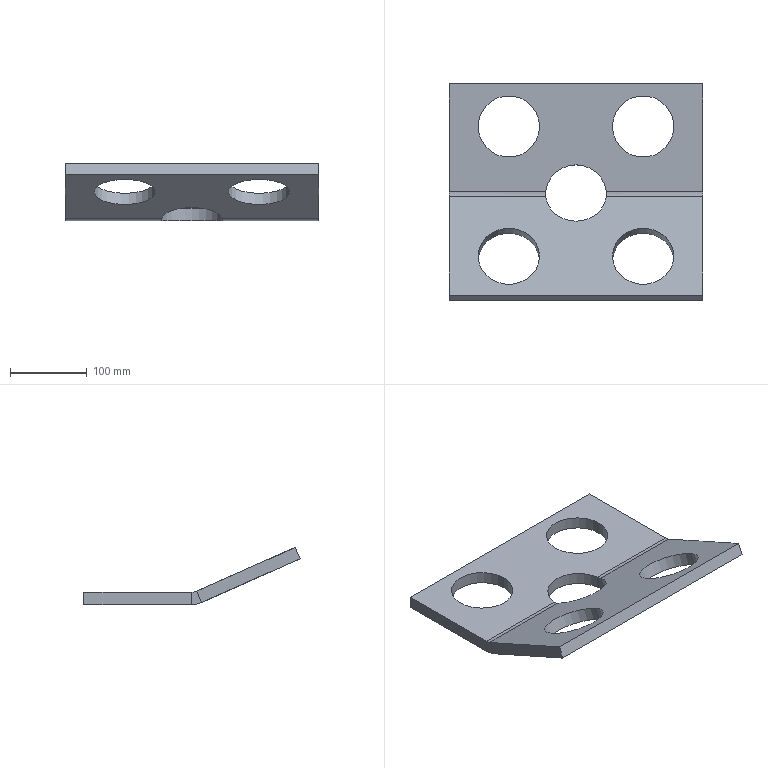Part | SolidWorks | features FlatPattern 1, SM3dBend 1, SMBaseFlange 1, SheetMetal 1 | 1 solid | 28 faces | box 330 x 281.818 x 74.519 mm | volume 1134363 mm3 | cylinder 14 | plane 12 | spline 2 | commonest cylinder face diameters 80 x10 32 x2 64 x2
STEP:
#1=CARTESIAN_POINT('',(212.5,235.5,-16.));
#2=VERTEX_POINT('',#1);
#3=CARTESIAN_POINT('',(292.5,235.5,-16.));
#4=VERTEX_POINT('',#3);
#5=CARTESIAN_POINT('',(252.5,235.5,-16.));
#6=DIRECTION('',(0.,0.,1.));
#7=DIRECTION('',(1.,0.,0.));
#8=AXIS2_PLACEMENT_3D('',#5,#6,#7);
#9=CIRCLE('',#8,40.);
#10=EDGE_CURVE('',#2,#4,#9,.T.);
#11=ORIENTED_EDGE('',*,*,#10,.F.);
#12=CARTESIAN_POINT('',(212.5,235.5,0.));
#13=VERTEX_POINT('',#12);
#14=CARTESIAN_POINT('',(212.5,235.5,-16.));
#15=DIRECTION('',(0.,0.,1.));
#16=VECTOR('',#15,1000.);
#17=LINE('',#14,#16);
#18=EDGE_CURVE('',#2,#13,#17,.T.);
#19=ORIENTED_EDGE('',*,*,#18,.T.);
#20=CARTESIAN_POINT('',(292.5,235.5,0.));
#21=VERTEX_POINT('',#20);
#22=CARTESIAN_POINT('',(252.5,235.5,0.));
#23=DIRECTION('',(0.,0.,1.));
#24=DIRECTION('',(1.,0.,0.));
#25=AXIS2_PLACEMENT_3D('',#22,#23,#24);
#26=CIRCLE('',#25,40.);
#27=EDGE_CURVE('',#13,#21,#26,.T.);
#28=ORIENTED_EDGE('',*,*,#27,.T.);
#29=CARTESIAN_POINT('',(292.5,235.5,-16.));
#30=DIRECTION('',(0.,0.,1.));
#31=VECTOR('',#30,1000.);
#32=LINE('',#29,#31);
#33=EDGE_CURVE('',#4,#21,#32,.T.);
#34=ORIENTED_EDGE('',*,*,#33,.F.);
#35=EDGE_LOOP('',(#11,#19,#28,#34));
#36=FACE_OUTER_BOUND('',#35,.T.);
#37=CARTESIAN_POINT('',(252.5,235.5,-16.));
#38=DIRECTION('',(0.,0.,1.));
#39=DIRECTION('',(1.,0.,0.));
#40=AXIS2_PLACEMENT_3D('',#37,#38,#39);
#41=CYLINDRICAL_SURFACE('',#40,40.);
#42=ADVANCED_FACE('',(#36),#41,.F.);
#43=CARTESIAN_POINT('',(37.5,235.5,-16.));
#44=VERTEX_POINT('',#43);
#45=CARTESIAN_POINT('',(117.5,235.5,-16.));
#46=VERTEX_POINT('',#45);
#47=CARTESIAN_POINT('',(77.5,235.5,-16.));
#48=DIRECTION('',(0.,0.,1.));
#49=DIRECTION('',(1.,0.,0.));
#50=AXIS2_PLACEMENT_3D('',#47,#48,#49);
#51=CIRCLE('',#50,40.);
#52=EDGE_CURVE('',#44,#46,#51,.T.);
#53=ORIENTED_EDGE('',*,*,#52,.F.);
#54=CARTESIAN_POINT('',(37.5,235.5,0.));
#55=VERTEX_POINT('',#54);
#56=CARTESIAN_POINT('',(37.5,235.5,-16.));
#57=DIRECTION('',(0.,0.,1.));
#58=VECTOR('',#57,1000.);
#59=LINE('',#56,#58);
#60=EDGE_CURVE('',#44,#55,#59,.T.);
#61=ORIENTED_EDGE('',*,*,#60,.T.);
#62=CARTESIAN_POINT('',(117.5,235.5,0.));
#63=VERTEX_POINT('',#62);
#64=CARTESIAN_POINT('',(77.5,235.5,0.));
#65=DIRECTION('',(0.,0.,1.));
#66=DIRECTION('',(1.,0.,0.));
#67=AXIS2_PLACEMENT_3D('',#64,#65,#66);
#68=CIRCLE('',#67,40.);
#69=EDGE_CURVE('',#55,#63,#68,.T.);
#70=ORIENTED_EDGE('',*,*,#69,.T.);
#71=CARTESIAN_POINT('',(117.5,235.5,-16.));
#72=DIRECTION('',(0.,0.,1.));
#73=VECTOR('',#72,1000.);
#74=LINE('',#71,#73);
#75=EDGE_CURVE('',#46,#63,#74,.T.);
#76=ORIENTED_EDGE('',*,*,#75,.F.);
#77=EDGE_LOOP('',(#53,#61,#70,#76));
#78=FACE_OUTER_BOUND('',#77,.T.);
#79=CARTESIAN_POINT('',(77.5,235.5,-16.));
#80=DIRECTION('',(0.,0.,1.));
#81=DIRECTION('',(1.,0.,0.));
#82=AXIS2_PLACEMENT_3D('',#79,#80,#81);
#83=CYLINDRICAL_SURFACE('',#82,40.);
#84=ADVANCED_FACE('',(#78),#83,.F.);
#85=CARTESIAN_POINT('',(212.5,59.884,21.328));
#86=VERTEX_POINT('',#85);
#87=CARTESIAN_POINT('',(292.5,59.884,21.328));
#88=VERTEX_POINT('',#87);
#89=CARTESIAN_POINT('',(252.5,59.884,21.328));
#90=DIRECTION('',(0.,0.4067,0.9135));
#91=DIRECTION('',(1.,0.,0.));
#92=AXIS2_PLACEMENT_3D('',#89,#90,#91);
#93=CIRCLE('',#92,40.);
#94=EDGE_CURVE('',#86,#88,#93,.T.);
#95=ORIENTED_EDGE('',*,*,#94,.F.);
#96=CARTESIAN_POINT('',(212.5,66.392,35.945));
#97=VERTEX_POINT('',#96);
#98=CARTESIAN_POINT('',(212.5,59.884,21.328));
#99=DIRECTION('',(0.,0.4067,0.9135));
#100=VECTOR('',#99,1000.);
#101=LINE('',#98,#100);
#102=EDGE_CURVE('',#86,#97,#101,.T.);
#103=ORIENTED_EDGE('',*,*,#102,.T.);
#104=CARTESIAN_POINT('',(292.5,66.392,35.945));
#105=VERTEX_POINT('',#104);
#106=CARTESIAN_POINT('',(252.5,66.392,35.945));
#107=DIRECTION('',(0.,0.4067,0.9135));
#108=DIRECTION('',(1.,0.,0.));
#109=AXIS2_PLACEMENT_3D('',#106,#107,#108);
#110=CIRCLE('',#109,40.);
#111=EDGE_CURVE('',#97,#105,#110,.T.);
#112=ORIENTED_EDGE('',*,*,#111,.T.);
#113=CARTESIAN_POINT('',(292.5,59.884,21.328));
#114=DIRECTION('',(0.,0.4067,0.9135));
#115=VECTOR('',#114,1000.);
#116=LINE('',#113,#115);
#117=EDGE_CURVE('',#88,#105,#116,.T.);
#118=ORIENTED_EDGE('',*,*,#117,.F.);
#119=EDGE_LOOP('',(#95,#103,#112,#118));
#120=FACE_OUTER_BOUND('',#119,.T.);
#121=CARTESIAN_POINT('',(252.5,59.884,21.328));
#122=DIRECTION('',(0.,0.4067,0.9135));
#123=DIRECTION('',(1.,0.,0.));
#124=AXIS2_PLACEMENT_3D('',#121,#122,#123);
#125=CYLINDRICAL_SURFACE('',#124,40.);
#126=ADVANCED_FACE('',(#120),#125,.F.);
#127=CARTESIAN_POINT('',(37.5,59.884,21.328));
#128=VERTEX_POINT('',#127);
#129=CARTESIAN_POINT('',(117.5,59.884,21.328));
#130=VERTEX_POINT('',#129);
#131=CARTESIAN_POINT('',(77.5,59.884,21.328));
#132=DIRECTION('',(0.,0.4067,0.9135));
#133=DIRECTION('',(1.,0.,0.));
#134=AXIS2_PLACEMENT_3D('',#131,#132,#133);
#135=CIRCLE('',#134,40.);
#136=EDGE_CURVE('',#128,#130,#135,.T.);
#137=ORIENTED_EDGE('',*,*,#136,.F.);
#138=CARTESIAN_POINT('',(37.5,66.392,35.945));
#139=VERTEX_POINT('',#138);
#140=CARTESIAN_POINT('',(37.5,59.884,21.328));
#141=DIRECTION('',(0.,0.4067,0.9135));
#142=VECTOR('',#141,1000.);
#143=LINE('',#140,#142);
#144=EDGE_CURVE('',#128,#139,#143,.T.);
#145=ORIENTED_EDGE('',*,*,#144,.T.);
#146=CARTESIAN_POINT('',(117.5,66.392,35.945));
#147=VERTEX_POINT('',#146);
#148=CARTESIAN_POINT('',(77.5,66.392,35.945));
#149=DIRECTION('',(0.,0.4067,0.9135));
#150=DIRECTION('',(1.,0.,0.));
#151=AXIS2_PLACEMENT_3D('',#148,#149,#150);
#152=CIRCLE('',#151,40.);
#153=EDGE_CURVE('',#139,#147,#152,.T.);
#154=ORIENTED_EDGE('',*,*,#153,.T.);
#155=CARTESIAN_POINT('',(117.5,59.884,21.328));
#156=DIRECTION('',(0.,0.4067,0.9135));
#157=VECTOR('',#156,1000.);
#158=LINE('',#155,#157);
#159=EDGE_CURVE('',#130,#147,#158,.T.);
#160=ORIENTED_EDGE('',*,*,#159,.F.);
#161=EDGE_LOOP('',(#137,#145,#154,#160));
#162=FACE_OUTER_BOUND('',#161,.T.);
#163=CARTESIAN_POINT('',(77.5,59.884,21.328));
#164=DIRECTION('',(0.,0.4067,0.9135));
#165=DIRECTION('',(1.,0.,0.));
#166=AXIS2_PLACEMENT_3D('',#163,#164,#165);
#167=CYLINDRICAL_SURFACE('',#166,40.);
#168=ADVANCED_FACE('',(#162),#167,.F.);
#169=CARTESIAN_POINT('',(0.,144.019,1.383));
#170=VERTEX_POINT('',#169);
#171=CARTESIAN_POINT('',(0.,15.69,58.519));
#172=VERTEX_POINT('',#171);
#173=CARTESIAN_POINT('',(0.,15.69,58.519));
#174=DIRECTION('',(0.,-0.9135,0.4067));
#175=VECTOR('',#174,1000.);
#176=LINE('',#173,#175);
#177=EDGE_CURVE('',#170,#172,#176,.T.);
#178=ORIENTED_EDGE('',*,*,#177,.F.);
#179=CARTESIAN_POINT('',(0.,137.511,-13.233));
#180=VERTEX_POINT('',#179);
#181=CARTESIAN_POINT('',(0.,137.511,-13.233));
#182=DIRECTION('',(0.,-0.4067,-0.9135));
#183=VECTOR('',#182,1000.);
#184=LINE('',#181,#183);
#185=EDGE_CURVE('',#170,#180,#184,.T.);
#186=ORIENTED_EDGE('',*,*,#185,.T.);
#187=CARTESIAN_POINT('',(0.,9.182,43.902));
#188=VERTEX_POINT('',#187);
#189=CARTESIAN_POINT('',(0.,9.182,43.902));
#190=DIRECTION('',(0.,-0.9135,0.4067));
#191=VECTOR('',#190,1000.);
#192=LINE('',#189,#191);
#193=EDGE_CURVE('',#180,#188,#192,.T.);
#194=ORIENTED_EDGE('',*,*,#193,.T.);
#195=CARTESIAN_POINT('',(0.,9.182,43.902));
#196=DIRECTION('',(0.,0.4067,0.9135));
#197=VECTOR('',#196,1000.);
#198=LINE('',#195,#197);
#199=EDGE_CURVE('',#188,#172,#198,.T.);
#200=ORIENTED_EDGE('',*,*,#199,.T.);
#201=EDGE_LOOP('',(#178,#186,#194,#200));
#202=FACE_OUTER_BOUND('',#201,.T.);
#203=CARTESIAN_POINT('',(0.,9.182,43.902));
#204=DIRECTION('',(-1.,0.,0.));
#205=DIRECTION('',(0.,0.4067,0.9135));
#206=AXIS2_PLACEMENT_3D('',#203,#204,#205);
#207=PLANE('',#206);
#208=ADVANCED_FACE('',(#202),#207,.T.);
#209=CARTESIAN_POINT('',(330.,9.182,43.902));
#210=VERTEX_POINT('',#209);
#211=CARTESIAN_POINT('',(330.,137.511,-13.233));
#212=VERTEX_POINT('',#211);
#213=CARTESIAN_POINT('',(330.,9.182,43.902));
#214=DIRECTION('',(0.,0.9135,-0.4067));
#215=VECTOR('',#214,1000.);
#216=LINE('',#213,#215);
#217=EDGE_CURVE('',#210,#212,#216,.T.);
#218=ORIENTED_EDGE('',*,*,#217,.T.);
#219=CARTESIAN_POINT('',(330.,144.019,1.383));
#220=VERTEX_POINT('',#219);
#221=CARTESIAN_POINT('',(330.,137.511,-13.233));
#222=DIRECTION('',(0.,0.4067,0.9135));
#223=VECTOR('',#222,1000.);
#224=LINE('',#221,#223);
#225=EDGE_CURVE('',#212,#220,#224,.T.);
#226=ORIENTED_EDGE('',*,*,#225,.T.);
#227=CARTESIAN_POINT('',(330.,15.69,58.519));
#228=VERTEX_POINT('',#227);
#229=CARTESIAN_POINT('',(330.,15.69,58.519));
#230=DIRECTION('',(0.,0.9135,-0.4067));
#231=VECTOR('',#230,1000.);
#232=LINE('',#229,#231);
#233=EDGE_CURVE('',#228,#220,#232,.T.);
#234=ORIENTED_EDGE('',*,*,#233,.F.);
#235=CARTESIAN_POINT('',(330.,9.182,43.902));
#236=DIRECTION('',(0.,0.4067,0.9135));
#237=VECTOR('',#236,1000.);
#238=LINE('',#235,#237);
#239=EDGE_CURVE('',#210,#228,#238,.T.);
#240=ORIENTED_EDGE('',*,*,#239,.F.);
#241=EDGE_LOOP('',(#218,#226,#234,#240));
#242=FACE_OUTER_BOUND('',#241,.T.);
#243=CARTESIAN_POINT('',(330.,9.182,43.902));
#244=DIRECTION('',(1.,0.,0.));
#245=DIRECTION('',(0.,-0.4067,-0.9135));
#246=AXIS2_PLACEMENT_3D('',#243,#244,#245);
#247=PLANE('',#246);
#248=ADVANCED_FACE('',(#242),#247,.T.);
#249=CARTESIAN_POINT('',(77.5,59.884,21.328));
#250=DIRECTION('',(0.,0.4067,0.9135));
#251=DIRECTION('',(1.,0.,0.));
#252=AXIS2_PLACEMENT_3D('',#249,#250,#251);
#253=CIRCLE('',#252,40.);
#254=EDGE_CURVE('',#130,#128,#253,.T.);
#255=ORIENTED_EDGE('',*,*,#254,.T.);
#256=ORIENTED_EDGE('',*,*,#136,.T.);
#257=EDGE_LOOP('',(#255,#256));
#258=FACE_BOUND('',#257,.T.);
#259=CARTESIAN_POINT('',(252.5,59.884,21.328));
#260=DIRECTION('',(0.,0.4067,0.9135));
#261=DIRECTION('',(1.,0.,0.));
#262=AXIS2_PLACEMENT_3D('',#259,#260,#261);
#263=CIRCLE('',#262,40.);
#264=EDGE_CURVE('',#88,#86,#263,.T.);
#265=ORIENTED_EDGE('',*,*,#264,.T.);
#266=ORIENTED_EDGE('',*,*,#94,.T.);
#267=EDGE_LOOP('',(#265,#266));
#268=FACE_BOUND('',#267,.T.);
#269=ORIENTED_EDGE('',*,*,#193,.F.);
#270=CARTESIAN_POINT('',(125.317,137.511,-13.233));
#271=VERTEX_POINT('',#270);
#272=CARTESIAN_POINT('',(0.,137.511,-13.233));
#273=DIRECTION('',(1.,0.,0.));
#274=VECTOR('',#273,1000.);
#275=LINE('',#272,#274);
#276=EDGE_CURVE('',#180,#271,#275,.T.);
#277=ORIENTED_EDGE('',*,*,#276,.T.);
#278=CARTESIAN_POINT('',(204.683,137.511,-13.233));
#279=VERTEX_POINT('',#278);
#280=CARTESIAN_POINT('',(165.,142.103,-15.278));
#281=DIRECTION('',(0.,0.4067,0.9135));
#282=DIRECTION('',(1.,0.,0.));
#283=AXIS2_PLACEMENT_3D('',#280,#281,#282);
#284=CIRCLE('',#283,40.);
#285=EDGE_CURVE('',#271,#279,#284,.T.);
#286=ORIENTED_EDGE('',*,*,#285,.T.);
#287=CARTESIAN_POINT('',(0.,137.511,-13.233));
#288=DIRECTION('',(1.,0.,0.));
#289=VECTOR('',#288,1000.);
#290=LINE('',#287,#289);
#291=EDGE_CURVE('',#279,#212,#290,.T.);
#292=ORIENTED_EDGE('',*,*,#291,.T.);
#293=ORIENTED_EDGE('',*,*,#217,.F.);
#294=CARTESIAN_POINT('',(0.,9.182,43.902));
#295=DIRECTION('',(1.,0.,0.));
#296=VECTOR('',#295,1000.);
#297=LINE('',#294,#296);
#298=EDGE_CURVE('',#188,#210,#297,.T.);
#299=ORIENTED_EDGE('',*,*,#298,.F.);
#300=EDGE_LOOP('',(#269,#277,#286,#292,#293,#299));
#301=FACE_OUTER_BOUND('',#300,.T.);
#302=CARTESIAN_POINT('',(0.,275.024,-74.458));
#303=DIRECTION('',(0.,-0.4067,-0.9135));
#304=DIRECTION('',(-1.,0.,0.));
#305=AXIS2_PLACEMENT_3D('',#302,#303,#304);
#306=PLANE('',#305);
#307=ADVANCED_FACE('',(#258,#268,#301),#306,.T.);
#308=CARTESIAN_POINT('',(0.,15.69,58.519));
#309=DIRECTION('',(1.,0.,0.));
#310=VECTOR('',#309,1000.);
#311=LINE('',#308,#310);
#312=EDGE_CURVE('',#172,#228,#311,.T.);
#313=ORIENTED_EDGE('',*,*,#312,.F.);
#314=ORIENTED_EDGE('',*,*,#199,.F.);
#315=ORIENTED_EDGE('',*,*,#298,.T.);
#316=ORIENTED_EDGE('',*,*,#239,.T.);
#317=EDGE_LOOP('',(#313,#314,#315,#316));
#318=FACE_OUTER_BOUND('',#317,.T.);
#319=CARTESIAN_POINT('',(0.,9.182,43.902));
#320=DIRECTION('',(0.,-0.9135,0.4067));
#321=DIRECTION('',(0.,-0.4067,-0.9135));
#322=AXIS2_PLACEMENT_3D('',#319,#320,#321);
#323=PLANE('',#322);
#324=ADVANCED_FACE('',(#318),#323,.T.);
#325=CARTESIAN_POINT('',(125.317,144.019,1.383));
#326=VERTEX_POINT('',#325);
#327=CARTESIAN_POINT('',(0.,144.019,1.383));
#328=DIRECTION('',(1.,0.,0.));
#329=VECTOR('',#328,1000.);
#330=LINE('',#327,#329);
#331=EDGE_CURVE('',#170,#326,#330,.T.);
#332=ORIENTED_EDGE('',*,*,#331,.F.);
#333=ORIENTED_EDGE('',*,*,#177,.T.);
#334=ORIENTED_EDGE('',*,*,#312,.T.);
#335=ORIENTED_EDGE('',*,*,#233,.T.);
#336=CARTESIAN_POINT('',(204.683,144.019,1.383));
#337=VERTEX_POINT('',#336);
#338=CARTESIAN_POINT('',(0.,144.019,1.383));
#339=DIRECTION('',(1.,0.,0.));
#340=VECTOR('',#339,1000.);
#341=LINE('',#338,#340);
#342=EDGE_CURVE('',#337,#220,#341,.T.);
#343=ORIENTED_EDGE('',*,*,#342,.F.);
#344=CARTESIAN_POINT('',(165.,148.611,-0.6612));
#345=DIRECTION('',(0.,0.4067,0.9135));
#346=DIRECTION('',(1.,0.,0.));
#347=AXIS2_PLACEMENT_3D('',#344,#345,#346);
#348=CIRCLE('',#347,40.);
#349=EDGE_CURVE('',#326,#337,#348,.T.);
#350=ORIENTED_EDGE('',*,*,#349,.F.);
#351=EDGE_LOOP('',(#332,#333,#334,#335,#343,#350));
#352=FACE_OUTER_BOUND('',#351,.T.);
#353=CARTESIAN_POINT('',(252.5,66.392,35.945));
#354=DIRECTION('',(0.,0.4067,0.9135));
#355=DIRECTION('',(1.,0.,0.));
#356=AXIS2_PLACEMENT_3D('',#353,#354,#355);
#357=CIRCLE('',#356,40.);
#358=EDGE_CURVE('',#105,#97,#357,.T.);
#359=ORIENTED_EDGE('',*,*,#358,.F.);
#360=ORIENTED_EDGE('',*,*,#111,.F.);
#361=EDGE_LOOP('',(#359,#360));
#362=FACE_BOUND('',#361,.T.);
#363=CARTESIAN_POINT('',(77.5,66.392,35.945));
#364=DIRECTION('',(0.,0.4067,0.9135));
#365=DIRECTION('',(1.,0.,0.));
#366=AXIS2_PLACEMENT_3D('',#363,#364,#365);
#367=CIRCLE('',#366,40.);
#368=EDGE_CURVE('',#147,#139,#367,.T.);
#369=ORIENTED_EDGE('',*,*,#368,.F.);
#370=ORIENTED_EDGE('',*,*,#153,.F.);
#371=EDGE_LOOP('',(#369,#370));
#372=FACE_BOUND('',#371,.T.);
#373=CARTESIAN_POINT('',(0.,281.532,-59.841));
#374=DIRECTION('',(0.,-0.4067,-0.9135));
#375=DIRECTION('',(-1.,0.,0.));
#376=AXIS2_PLACEMENT_3D('',#373,#374,#375);
#377=PLANE('',#376);
#378=ADVANCED_FACE('',(#352,#362,#372),#377,.F.);
#379=CARTESIAN_POINT('',(125.317,144.019,1.383));
#380=CARTESIAN_POINT('',(125.317,137.511,-13.233));
#381=B_SPLINE_CURVE_WITH_KNOTS('',1,(#379,#380),.UNSPECIFIED.,.F.,.F.,(2,2),(0.,1.),.UNSPECIFIED.);
#382=EDGE_CURVE('',#326,#271,#381,.T.);
#383=ORIENTED_EDGE('',*,*,#382,.F.);
#384=ORIENTED_EDGE('',*,*,#349,.T.);
#385=CARTESIAN_POINT('',(204.683,137.511,-13.233));
#386=CARTESIAN_POINT('',(204.683,144.019,1.383));
#387=B_SPLINE_CURVE_WITH_KNOTS('',1,(#385,#386),.UNSPECIFIED.,.F.,.F.,(2,2),(0.,1.),.UNSPECIFIED.);
#388=EDGE_CURVE('',#279,#337,#387,.T.);
#389=ORIENTED_EDGE('',*,*,#388,.F.);
#390=ORIENTED_EDGE('',*,*,#285,.F.);
#391=EDGE_LOOP('',(#383,#384,#389,#390));
#392=FACE_OUTER_BOUND('',#391,.T.);
#393=CARTESIAN_POINT('',(165.,142.103,-15.278));
#394=DIRECTION('',(0.,0.4067,0.9135));
#395=DIRECTION('',(1.,0.,0.));
#396=AXIS2_PLACEMENT_3D('',#393,#394,#395);
#397=CYLINDRICAL_SURFACE('',#396,40.);
#398=ADVANCED_FACE('',(#392),#397,.F.);
#399=ORIENTED_EDGE('',*,*,#144,.F.);
#400=ORIENTED_EDGE('',*,*,#254,.F.);
#401=ORIENTED_EDGE('',*,*,#159,.T.);
#402=ORIENTED_EDGE('',*,*,#368,.T.);
#403=EDGE_LOOP('',(#399,#400,#401,#402));
#404=FACE_OUTER_BOUND('',#403,.T.);
#405=CARTESIAN_POINT('',(77.5,59.884,21.328));
#406=DIRECTION('',(0.,0.4067,0.9135));
#407=DIRECTION('',(1.,0.,0.));
#408=AXIS2_PLACEMENT_3D('',#405,#406,#407);
#409=CYLINDRICAL_SURFACE('',#408,40.);
#410=ADVANCED_FACE('',(#404),#409,.F.);
#411=ORIENTED_EDGE('',*,*,#102,.F.);
#412=ORIENTED_EDGE('',*,*,#264,.F.);
#413=ORIENTED_EDGE('',*,*,#117,.T.);
#414=ORIENTED_EDGE('',*,*,#358,.T.);
#415=EDGE_LOOP('',(#411,#412,#413,#414));
#416=FACE_OUTER_BOUND('',#415,.T.);
#417=CARTESIAN_POINT('',(252.5,59.884,21.328));
#418=DIRECTION('',(0.,0.4067,0.9135));
#419=DIRECTION('',(1.,0.,0.));
#420=AXIS2_PLACEMENT_3D('',#417,#418,#419);
#421=CYLINDRICAL_SURFACE('',#420,40.);
#422=ADVANCED_FACE('',(#416),#421,.F.);
#423=ORIENTED_EDGE('',*,*,#60,.F.);
#424=CARTESIAN_POINT('',(77.5,235.5,-16.));
#425=DIRECTION('',(0.,0.,1.));
#426=DIRECTION('',(1.,0.,0.));
#427=AXIS2_PLACEMENT_3D('',#424,#425,#426);
#428=CIRCLE('',#427,40.);
#429=EDGE_CURVE('',#46,#44,#428,.T.);
#430=ORIENTED_EDGE('',*,*,#429,.F.);
#431=ORIENTED_EDGE('',*,*,#75,.T.);
#432=CARTESIAN_POINT('',(77.5,235.5,0.));
#433=DIRECTION('',(0.,0.,1.));
#434=DIRECTION('',(1.,0.,0.));
#435=AXIS2_PLACEMENT_3D('',#432,#433,#434);
#436=CIRCLE('',#435,40.);
#437=EDGE_CURVE('',#63,#55,#436,.T.);
#438=ORIENTED_EDGE('',*,*,#437,.T.);
#439=EDGE_LOOP('',(#423,#430,#431,#438));
#440=FACE_OUTER_BOUND('',#439,.T.);
#441=CARTESIAN_POINT('',(77.5,235.5,-16.));
#442=DIRECTION('',(0.,0.,1.));
#443=DIRECTION('',(1.,0.,0.));
#444=AXIS2_PLACEMENT_3D('',#441,#442,#443);
#445=CYLINDRICAL_SURFACE('',#444,40.);
#446=ADVANCED_FACE('',(#440),#445,.F.);
#447=ORIENTED_EDGE('',*,*,#18,.F.);
#448=CARTESIAN_POINT('',(252.5,235.5,-16.));
#449=DIRECTION('',(0.,0.,1.));
#450=DIRECTION('',(1.,0.,0.));
#451=AXIS2_PLACEMENT_3D('',#448,#449,#450);
#452=CIRCLE('',#451,40.);
#453=EDGE_CURVE('',#4,#2,#452,.T.);
#454=ORIENTED_EDGE('',*,*,#453,.F.);
#455=ORIENTED_EDGE('',*,*,#33,.T.);
#456=CARTESIAN_POINT('',(252.5,235.5,0.));
#457=DIRECTION('',(0.,0.,1.));
#458=DIRECTION('',(1.,0.,0.));
#459=AXIS2_PLACEMENT_3D('',#456,#457,#458);
#460=CIRCLE('',#459,40.);
#461=EDGE_CURVE('',#21,#13,#460,.T.);
#462=ORIENTED_EDGE('',*,*,#461,.T.);
#463=EDGE_LOOP('',(#447,#454,#455,#462));
#464=FACE_OUTER_BOUND('',#463,.T.);
#465=CARTESIAN_POINT('',(252.5,235.5,-16.));
#466=DIRECTION('',(0.,0.,1.));
#467=DIRECTION('',(1.,0.,0.));
#468=AXIS2_PLACEMENT_3D('',#465,#466,#467);
#469=CYLINDRICAL_SURFACE('',#468,40.);
#470=ADVANCED_FACE('',(#464),#469,.F.);
#471=CARTESIAN_POINT('',(330.,291.,0.));
#472=VERTEX_POINT('',#471);
#473=CARTESIAN_POINT('',(0.,291.,0.));
#474=VERTEX_POINT('',#473);
#475=CARTESIAN_POINT('',(0.,291.,0.));
#476=DIRECTION('',(-1.,0.,0.));
#477=VECTOR('',#476,1000.);
#478=LINE('',#475,#477);
#479=EDGE_CURVE('',#472,#474,#478,.T.);
#480=ORIENTED_EDGE('',*,*,#479,.F.);
#481=CARTESIAN_POINT('',(330.,291.,-16.));
#482=VERTEX_POINT('',#481);
#483=CARTESIAN_POINT('',(330.,291.,-16.));
#484=DIRECTION('',(0.,0.,1.));
#485=VECTOR('',#484,1000.);
#486=LINE('',#483,#485);
#487=EDGE_CURVE('',#482,#472,#486,.T.);
#488=ORIENTED_EDGE('',*,*,#487,.F.);
#489=CARTESIAN_POINT('',(0.,291.,-16.));
#490=VERTEX_POINT('',#489);
#491=CARTESIAN_POINT('',(0.,291.,-16.));
#492=DIRECTION('',(-1.,0.,0.));
#493=VECTOR('',#492,1000.);
#494=LINE('',#491,#493);
#495=EDGE_CURVE('',#482,#490,#494,.T.);
#496=ORIENTED_EDGE('',*,*,#495,.T.);
#497=CARTESIAN_POINT('',(0.,291.,-16.));
#498=DIRECTION('',(0.,0.,1.));
#499=VECTOR('',#498,1000.);
#500=LINE('',#497,#499);
#501=EDGE_CURVE('',#490,#474,#500,.T.);
#502=ORIENTED_EDGE('',*,*,#501,.T.);
#503=EDGE_LOOP('',(#480,#488,#496,#502));
#504=FACE_OUTER_BOUND('',#503,.T.);
#505=CARTESIAN_POINT('',(0.,291.,-16.));
#506=DIRECTION('',(0.,1.,0.));
#507=DIRECTION('',(0.,0.,1.));
#508=AXIS2_PLACEMENT_3D('',#505,#506,#507);
#509=PLANE('',#508);
#510=ADVANCED_FACE('',(#504),#509,.T.);
#511=CARTESIAN_POINT('',(0.,150.527,-16.));
#512=VERTEX_POINT('',#511);
#513=CARTESIAN_POINT('',(125.317,150.527,-16.));
#514=VERTEX_POINT('',#513);
#515=CARTESIAN_POINT('',(0.,150.527,-16.));
#516=DIRECTION('',(1.,0.,0.));
#517=VECTOR('',#516,1000.);
#518=LINE('',#515,#517);
#519=EDGE_CURVE('',#512,#514,#518,.T.);
#520=ORIENTED_EDGE('',*,*,#519,.F.);
#521=CARTESIAN_POINT('',(0.,0.,-16.));
#522=DIRECTION('',(0.,-1.,0.));
#523=VECTOR('',#522,1000.);
#524=LINE('',#521,#523);
#525=EDGE_CURVE('',#490,#512,#524,.T.);
#526=ORIENTED_EDGE('',*,*,#525,.F.);
#527=ORIENTED_EDGE('',*,*,#495,.F.);
#528=CARTESIAN_POINT('',(330.,150.527,-16.));
#529=VERTEX_POINT('',#528);
#530=CARTESIAN_POINT('',(330.,0.,-16.));
#531=DIRECTION('',(0.,1.,0.));
#532=VECTOR('',#531,1000.);
#533=LINE('',#530,#532);
#534=EDGE_CURVE('',#529,#482,#533,.T.);
#535=ORIENTED_EDGE('',*,*,#534,.F.);
#536=CARTESIAN_POINT('',(204.683,150.527,-16.));
#537=VERTEX_POINT('',#536);
#538=CARTESIAN_POINT('',(0.,150.527,-16.));
#539=DIRECTION('',(1.,0.,0.));
#540=VECTOR('',#539,1000.);
#541=LINE('',#538,#540);
#542=EDGE_CURVE('',#537,#529,#541,.T.);
#543=ORIENTED_EDGE('',*,*,#542,.F.);
#544=CARTESIAN_POINT('',(165.,145.5,-16.));
#545=DIRECTION('',(0.,0.,1.));
#546=DIRECTION('',(1.,0.,0.));
#547=AXIS2_PLACEMENT_3D('',#544,#545,#546);
#548=CIRCLE('',#547,40.);
#549=EDGE_CURVE('',#537,#514,#548,.T.);
#550=ORIENTED_EDGE('',*,*,#549,.T.);
#551=EDGE_LOOP('',(#520,#526,#527,#535,#543,#550));
#552=FACE_OUTER_BOUND('',#551,.T.);
#553=ORIENTED_EDGE('',*,*,#453,.T.);
#554=ORIENTED_EDGE('',*,*,#10,.T.);
#555=EDGE_LOOP('',(#553,#554));
#556=FACE_BOUND('',#555,.T.);
#557=ORIENTED_EDGE('',*,*,#429,.T.);
#558=ORIENTED_EDGE('',*,*,#52,.T.);
#559=EDGE_LOOP('',(#557,#558));
#560=FACE_BOUND('',#559,.T.);
#561=CARTESIAN_POINT('',(0.,291.,-16.));
#562=DIRECTION('',(0.,0.,-1.));
#563=DIRECTION('',(-1.,0.,0.));
#564=AXIS2_PLACEMENT_3D('',#561,#562,#563);
#565=PLANE('',#564);
#566=ADVANCED_FACE('',(#552,#556,#560),#565,.T.);
#567=CARTESIAN_POINT('',(0.,150.527,0.));
#568=VERTEX_POINT('',#567);
#569=CARTESIAN_POINT('',(0.,150.527,-16.));
#570=DIRECTION('',(0.,0.,-1.));
#571=VECTOR('',#570,1000.);
#572=LINE('',#569,#571);
#573=EDGE_CURVE('',#568,#512,#572,.T.);
#574=ORIENTED_EDGE('',*,*,#573,.F.);
#575=CARTESIAN_POINT('',(0.,0.,0.));
#576=DIRECTION('',(0.,-1.,0.));
#577=VECTOR('',#576,1000.);
#578=LINE('',#575,#577);
#579=EDGE_CURVE('',#474,#568,#578,.T.);
#580=ORIENTED_EDGE('',*,*,#579,.F.);
#581=ORIENTED_EDGE('',*,*,#501,.F.);
#582=ORIENTED_EDGE('',*,*,#525,.T.);
#583=EDGE_LOOP('',(#574,#580,#581,#582));
#584=FACE_OUTER_BOUND('',#583,.T.);
#585=CARTESIAN_POINT('',(0.,0.,-16.));
#586=DIRECTION('',(-1.,0.,0.));
#587=DIRECTION('',(0.,0.,1.));
#588=AXIS2_PLACEMENT_3D('',#585,#586,#587);
#589=PLANE('',#588);
#590=ADVANCED_FACE('',(#584),#589,.T.);
#591=ORIENTED_EDGE('',*,*,#437,.F.);
#592=ORIENTED_EDGE('',*,*,#69,.F.);
#593=EDGE_LOOP('',(#591,#592));
#594=FACE_BOUND('',#593,.T.);
#595=ORIENTED_EDGE('',*,*,#461,.F.);
#596=ORIENTED_EDGE('',*,*,#27,.F.);
#597=EDGE_LOOP('',(#595,#596));
#598=FACE_BOUND('',#597,.T.);
#599=ORIENTED_EDGE('',*,*,#579,.T.);
#600=CARTESIAN_POINT('',(125.317,150.527,0.));
#601=VERTEX_POINT('',#600);
#602=CARTESIAN_POINT('',(0.,150.527,0.));
#603=DIRECTION('',(1.,0.,0.));
#604=VECTOR('',#603,1000.);
#605=LINE('',#602,#604);
#606=EDGE_CURVE('',#568,#601,#605,.T.);
#607=ORIENTED_EDGE('',*,*,#606,.T.);
#608=CARTESIAN_POINT('',(204.683,150.527,0.));
#609=VERTEX_POINT('',#608);
#610=CARTESIAN_POINT('',(165.,145.5,0.));
#611=DIRECTION('',(0.,0.,1.));
#612=DIRECTION('',(1.,0.,0.));
#613=AXIS2_PLACEMENT_3D('',#610,#611,#612);
#614=CIRCLE('',#613,40.);
#615=EDGE_CURVE('',#609,#601,#614,.T.);
#616=ORIENTED_EDGE('',*,*,#615,.F.);
#617=CARTESIAN_POINT('',(330.,150.527,0.));
#618=VERTEX_POINT('',#617);
#619=CARTESIAN_POINT('',(0.,150.527,0.));
#620=DIRECTION('',(1.,0.,0.));
#621=VECTOR('',#620,1000.);
#622=LINE('',#619,#621);
#623=EDGE_CURVE('',#609,#618,#622,.T.);
#624=ORIENTED_EDGE('',*,*,#623,.T.);
#625=CARTESIAN_POINT('',(330.,0.,0.));
#626=DIRECTION('',(0.,1.,0.));
#627=VECTOR('',#626,1000.);
#628=LINE('',#625,#627);
#629=EDGE_CURVE('',#618,#472,#628,.T.);
#630=ORIENTED_EDGE('',*,*,#629,.T.);
#631=ORIENTED_EDGE('',*,*,#479,.T.);
#632=EDGE_LOOP('',(#599,#607,#616,#624,#630,#631));
#633=FACE_OUTER_BOUND('',#632,.T.);
#634=CARTESIAN_POINT('',(0.,291.,0.));
#635=DIRECTION('',(0.,0.,-1.));
#636=DIRECTION('',(-1.,0.,0.));
#637=AXIS2_PLACEMENT_3D('',#634,#635,#636);
#638=PLANE('',#637);
#639=ADVANCED_FACE('',(#594,#598,#633),#638,.F.);
#640=ORIENTED_EDGE('',*,*,#615,.T.);
#641=CARTESIAN_POINT('',(125.317,150.527,0.));
#642=CARTESIAN_POINT('',(125.317,150.527,-5.333));
#643=CARTESIAN_POINT('',(125.317,150.527,-10.667));
#644=CARTESIAN_POINT('',(125.317,150.527,-16.));
#645=B_SPLINE_CURVE_WITH_KNOTS('',3,(#641,#642,#643,#644),.UNSPECIFIED.,.F.,.F.,(4,4),(0.,1.),.UNSPECIFIED.);
#646=EDGE_CURVE('',#601,#514,#645,.T.);
#647=ORIENTED_EDGE('',*,*,#646,.T.);
#648=ORIENTED_EDGE('',*,*,#549,.F.);
#649=CARTESIAN_POINT('',(204.683,150.527,-16.));
#650=CARTESIAN_POINT('',(204.683,150.527,-10.667));
#651=CARTESIAN_POINT('',(204.683,150.527,-5.333));
#652=CARTESIAN_POINT('',(204.683,150.527,0.));
#653=B_SPLINE_CURVE_WITH_KNOTS('',3,(#649,#650,#651,#652),.UNSPECIFIED.,.F.,.F.,(4,4),(0.,1.),.UNSPECIFIED.);
#654=EDGE_CURVE('',#537,#609,#653,.T.);
#655=ORIENTED_EDGE('',*,*,#654,.T.);
#656=EDGE_LOOP('',(#640,#647,#648,#655));
#657=FACE_OUTER_BOUND('',#656,.T.);
#658=CARTESIAN_POINT('',(165.,145.5,-16.));
#659=DIRECTION('',(0.,0.,1.));
#660=DIRECTION('',(1.,0.,0.));
#661=AXIS2_PLACEMENT_3D('',#658,#659,#660);
#662=CYLINDRICAL_SURFACE('',#661,40.);
#663=ADVANCED_FACE('',(#657),#662,.F.);
#664=CARTESIAN_POINT('',(330.,150.527,-16.));
#665=DIRECTION('',(0.,0.,1.));
#666=VECTOR('',#665,1000.);
#667=LINE('',#664,#666);
#668=EDGE_CURVE('',#529,#618,#667,.T.);
#669=ORIENTED_EDGE('',*,*,#668,.F.);
#670=ORIENTED_EDGE('',*,*,#534,.T.);
#671=ORIENTED_EDGE('',*,*,#487,.T.);
#672=ORIENTED_EDGE('',*,*,#629,.F.);
#673=EDGE_LOOP('',(#669,#670,#671,#672));
#674=FACE_OUTER_BOUND('',#673,.T.);
#675=CARTESIAN_POINT('',(330.,0.,-16.));
#676=DIRECTION('',(1.,0.,0.));
#677=DIRECTION('',(0.,0.,-1.));
#678=AXIS2_PLACEMENT_3D('',#675,#676,#677);
#679=PLANE('',#678);
#680=ADVANCED_FACE('',(#674),#679,.T.);
#681=ORIENTED_EDGE('',*,*,#185,.F.);
#682=CARTESIAN_POINT('',(0.,150.527,16.));
#683=DIRECTION('',(1.,0.,0.));
#684=DIRECTION('',(0.,0.,1.));
#685=AXIS2_PLACEMENT_3D('',#682,#683,#684);
#686=CIRCLE('',#685,16.);
#687=EDGE_CURVE('',#170,#568,#686,.T.);
#688=ORIENTED_EDGE('',*,*,#687,.T.);
#689=ORIENTED_EDGE('',*,*,#573,.T.);
#690=CARTESIAN_POINT('',(0.,150.527,16.));
#691=DIRECTION('',(1.,0.,0.));
#692=DIRECTION('',(0.,0.,1.));
#693=AXIS2_PLACEMENT_3D('',#690,#691,#692);
#694=CIRCLE('',#693,32.);
#695=EDGE_CURVE('',#180,#512,#694,.T.);
#696=ORIENTED_EDGE('',*,*,#695,.F.);
#697=EDGE_LOOP('',(#681,#688,#689,#696));
#698=FACE_OUTER_BOUND('',#697,.T.);
#699=CARTESIAN_POINT('',(0.,150.527,16.));
#700=DIRECTION('',(-1.,0.,0.));
#701=DIRECTION('',(0.,0.,1.));
#702=AXIS2_PLACEMENT_3D('',#699,#700,#701);
#703=PLANE('',#702);
#704=ADVANCED_FACE('',(#698),#703,.T.);
#705=ORIENTED_EDGE('',*,*,#519,.T.);
#706=CARTESIAN_POINT('',(125.317,150.527,-16.));
#707=CARTESIAN_POINT('',(125.211,149.069,-16.));
#708=CARTESIAN_POINT('',(125.131,147.782,-15.902));
#709=CARTESIAN_POINT('',(125.051,146.119,-15.7));
#710=CARTESIAN_POINT('',(125.03,145.609,-15.623));
#711=CARTESIAN_POINT('',(125.009,144.909,-15.504));
#712=CARTESIAN_POINT('',(125.004,144.687,-15.463));
#713=CARTESIAN_POINT('',(124.998,144.369,-15.402));
#714=CARTESIAN_POINT('',(124.996,144.215,-15.372));
#715=CARTESIAN_POINT('',(124.994,144.042,-15.336));
#716=CARTESIAN_POINT('',(124.994,143.957,-15.318));
#717=CARTESIAN_POINT('',(124.994,143.921,-15.311));
#718=CARTESIAN_POINT('',(124.993,143.897,-15.306));
#719=CARTESIAN_POINT('',(124.993,143.887,-15.304));
#720=CARTESIAN_POINT('',(124.991,142.997,-15.114));
#721=CARTESIAN_POINT('',(125.017,142.019,-14.869));
#722=CARTESIAN_POINT('',(125.125,139.888,-14.2));
#723=CARTESIAN_POINT('',(125.207,138.733,-13.778));
#724=CARTESIAN_POINT('',(125.317,137.511,-13.233));
#725=B_SPLINE_CURVE_WITH_KNOTS('',3,(#706,#707,#708,#709,#710,#711,#712,#713,#714,#715,#716,#717,#718,#719,#720,#721,#722,#723,#724),.UNSPECIFIED.,.F.,.F.,(4,2,2,2,1,1,1,2,2,2,4),(0.,0.25,0.375,0.4375,0.4688,0.4844,0.4922,0.4961,0.5,0.75,1.),.UNSPECIFIED.);
#726=EDGE_CURVE('',#514,#271,#725,.T.);
#727=ORIENTED_EDGE('',*,*,#726,.T.);
#728=ORIENTED_EDGE('',*,*,#276,.F.);
#729=ORIENTED_EDGE('',*,*,#695,.T.);
#730=EDGE_LOOP('',(#705,#727,#728,#729));
#731=FACE_OUTER_BOUND('',#730,.T.);
#732=CARTESIAN_POINT('',(189.392,150.527,16.));
#733=DIRECTION('',(-1.,0.,0.));
#734=DIRECTION('',(0.,0.,1.));
#735=AXIS2_PLACEMENT_3D('',#732,#733,#734);
#736=CYLINDRICAL_SURFACE('',#735,32.);
#737=ADVANCED_FACE('',(#731),#736,.T.);
#738=CARTESIAN_POINT('',(125.317,150.527,0.));
#739=CARTESIAN_POINT('',(125.211,149.797,0.));
#740=CARTESIAN_POINT('',(125.131,149.154,0.04916));
#741=CARTESIAN_POINT('',(125.051,148.323,0.15));
#742=CARTESIAN_POINT('',(125.03,148.068,0.1883));
#743=CARTESIAN_POINT('',(125.009,147.718,0.248));
#744=CARTESIAN_POINT('',(125.004,147.607,0.2683));
#745=CARTESIAN_POINT('',(124.998,147.448,0.2989));
#746=CARTESIAN_POINT('',(124.996,147.396,0.3091));
#747=CARTESIAN_POINT('',(124.994,147.296,0.3294));
#748=CARTESIAN_POINT('',(124.994,147.255,0.338));
#749=CARTESIAN_POINT('',(124.988,146.323,0.536));
#750=CARTESIAN_POINT('',(125.096,145.242,0.8385));
#751=CARTESIAN_POINT('',(125.317,144.019,1.383));
#752=B_SPLINE_CURVE_WITH_KNOTS('',3,(#738,#739,#740,#741,#742,#743,#744,#745,#746,#747,#748,#749,#750,#751),.UNSPECIFIED.,.F.,.F.,(4,2,2,2,2,2,4),(0.,0.25,0.375,0.4375,0.4688,0.5,1.),.UNSPECIFIED.);
#753=EDGE_CURVE('',#601,#326,#752,.T.);
#754=ORIENTED_EDGE('',*,*,#753,.T.);
#755=ORIENTED_EDGE('',*,*,#382,.T.);
#756=ORIENTED_EDGE('',*,*,#726,.F.);
#757=ORIENTED_EDGE('',*,*,#646,.F.);
#758=EDGE_LOOP('',(#754,#755,#756,#757));
#759=FACE_OUTER_BOUND('',#758,.T.);
#760=CARTESIAN_POINT('',(125.317,150.527,-16.));
#761=CARTESIAN_POINT('',(125.211,149.068,-16.));
#762=CARTESIAN_POINT('',(125.131,147.782,-15.902));
#763=CARTESIAN_POINT('',(125.051,146.119,-15.7));
#764=CARTESIAN_POINT('',(125.03,145.609,-15.623));
#765=CARTESIAN_POINT('',(125.009,144.909,-15.504));
#766=CARTESIAN_POINT('',(125.004,144.687,-15.463));
#767=CARTESIAN_POINT('',(124.998,144.369,-15.402));
#768=CARTESIAN_POINT('',(124.996,144.266,-15.382));
#769=CARTESIAN_POINT('',(124.994,144.066,-15.341));
#770=CARTESIAN_POINT('',(124.994,143.983,-15.324));
#771=CARTESIAN_POINT('',(124.988,142.12,-14.928));
#772=CARTESIAN_POINT('',(125.096,139.958,-14.323));
#773=CARTESIAN_POINT('',(125.317,137.511,-13.233));
#774=CARTESIAN_POINT('',(125.317,150.527,0.));
#775=CARTESIAN_POINT('',(125.211,149.797,0.));
#776=CARTESIAN_POINT('',(125.131,149.154,0.04916));
#777=CARTESIAN_POINT('',(125.051,148.323,0.15));
#778=CARTESIAN_POINT('',(125.03,148.068,0.1883));
#779=CARTESIAN_POINT('',(125.009,147.718,0.248));
#780=CARTESIAN_POINT('',(125.004,147.607,0.2683));
#781=CARTESIAN_POINT('',(124.998,147.448,0.2989));
#782=CARTESIAN_POINT('',(124.996,147.396,0.3091));
#783=CARTESIAN_POINT('',(124.994,147.296,0.3294));
#784=CARTESIAN_POINT('',(124.994,147.255,0.338));
#785=CARTESIAN_POINT('',(124.988,146.323,0.536));
#786=CARTESIAN_POINT('',(125.096,145.242,0.8385));
#787=CARTESIAN_POINT('',(125.317,144.019,1.383));
#788=B_SPLINE_SURFACE_WITH_KNOTS('',1,3,((#760,#761,#762,#763,#764,#765,#766,#767,#768,#769,#770,#771,#772,#773),(#774,#775,#776,#777,#778,#779,#780,#781,#782,#783,#784,#785,#786,#787)),.UNSPECIFIED.,.F.,.F.,.F.,(2,2),(4,2,2,2,2,2,4),(0.,1.),(0.,0.25,0.375,0.4375,0.4688,0.5,1.),.UNSPECIFIED.);
#789=ADVANCED_FACE('',(#759),#788,.T.);
#790=ORIENTED_EDGE('',*,*,#606,.F.);
#791=ORIENTED_EDGE('',*,*,#687,.F.);
#792=ORIENTED_EDGE('',*,*,#331,.T.);
#793=ORIENTED_EDGE('',*,*,#753,.F.);
#794=EDGE_LOOP('',(#790,#791,#792,#793));
#795=FACE_OUTER_BOUND('',#794,.T.);
#796=CARTESIAN_POINT('',(189.392,150.527,16.));
#797=DIRECTION('',(-1.,0.,0.));
#798=DIRECTION('',(0.,0.,1.));
#799=AXIS2_PLACEMENT_3D('',#796,#797,#798);
#800=CYLINDRICAL_SURFACE('',#799,16.);
#801=ADVANCED_FACE('',(#795),#800,.F.);
#802=ORIENTED_EDGE('',*,*,#388,.T.);
#803=CARTESIAN_POINT('',(204.683,144.019,1.383));
#804=CARTESIAN_POINT('',(204.789,144.685,1.087));
#805=CARTESIAN_POINT('',(204.869,145.292,0.8701));
#806=CARTESIAN_POINT('',(204.949,146.093,0.624));
#807=CARTESIAN_POINT('',(204.97,146.342,0.5552));
#808=CARTESIAN_POINT('',(204.991,146.686,0.4674));
#809=CARTESIAN_POINT('',(204.996,146.795,0.4407));
#810=CARTESIAN_POINT('',(205.002,146.953,0.4041));
#811=CARTESIAN_POINT('',(205.004,147.004,0.3925));
#812=CARTESIAN_POINT('',(205.006,147.104,0.3703));
#813=CARTESIAN_POINT('',(205.006,147.145,0.3613));
#814=CARTESIAN_POINT('',(205.012,148.077,0.1633));
#815=CARTESIAN_POINT('',(204.904,149.187,0.));
#816=CARTESIAN_POINT('',(204.683,150.527,0.));
#817=B_SPLINE_CURVE_WITH_KNOTS('',3,(#803,#804,#805,#806,#807,#808,#809,#810,#811,#812,#813,#814,#815,#816),.UNSPECIFIED.,.F.,.F.,(4,2,2,2,2,2,4),(0.,0.25,0.375,0.4375,0.4688,0.5,1.),.UNSPECIFIED.);
#818=EDGE_CURVE('',#337,#609,#817,.T.);
#819=ORIENTED_EDGE('',*,*,#818,.T.);
#820=ORIENTED_EDGE('',*,*,#654,.F.);
#821=CARTESIAN_POINT('',(204.683,137.511,-13.233));
#822=CARTESIAN_POINT('',(204.789,138.843,-13.826));
#823=CARTESIAN_POINT('',(204.869,140.058,-14.26));
#824=CARTESIAN_POINT('',(204.949,141.659,-14.752));
#825=CARTESIAN_POINT('',(204.97,142.157,-14.89));
#826=CARTESIAN_POINT('',(204.991,142.845,-15.065));
#827=CARTESIAN_POINT('',(204.996,143.064,-15.119));
#828=CARTESIAN_POINT('',(205.002,143.379,-15.192));
#829=CARTESIAN_POINT('',(205.004,143.533,-15.227));
#830=CARTESIAN_POINT('',(205.006,143.705,-15.265));
#831=CARTESIAN_POINT('',(205.006,143.79,-15.283));
#832=CARTESIAN_POINT('',(205.006,143.826,-15.291));
#833=CARTESIAN_POINT('',(205.007,143.85,-15.296));
#834=CARTESIAN_POINT('',(205.007,143.86,-15.298));
#835=CARTESIAN_POINT('',(205.009,144.75,-15.487));
#836=CARTESIAN_POINT('',(204.983,145.743,-15.66));
#837=CARTESIAN_POINT('',(204.875,147.962,-15.917));
#838=CARTESIAN_POINT('',(204.793,149.189,-16.));
#839=CARTESIAN_POINT('',(204.683,150.527,-16.));
#840=B_SPLINE_CURVE_WITH_KNOTS('',3,(#821,#822,#823,#824,#825,#826,#827,#828,#829,#830,#831,#832,#833,#834,#835,#836,#837,#838,#839),.UNSPECIFIED.,.F.,.F.,(4,2,2,2,1,1,1,2,2,2,4),(0.,0.25,0.375,0.4375,0.4688,0.4844,0.4922,0.4961,0.5,0.75,1.),.UNSPECIFIED.);
#841=EDGE_CURVE('',#279,#537,#840,.T.);
#842=ORIENTED_EDGE('',*,*,#841,.F.);
#843=EDGE_LOOP('',(#802,#819,#820,#842));
#844=FACE_OUTER_BOUND('',#843,.T.);
#845=CARTESIAN_POINT('',(204.683,137.511,-13.233));
#846=CARTESIAN_POINT('',(204.789,138.843,-13.827));
#847=CARTESIAN_POINT('',(204.869,140.058,-14.26));
#848=CARTESIAN_POINT('',(204.949,141.659,-14.752));
#849=CARTESIAN_POINT('',(204.97,142.157,-14.89));
#850=CARTESIAN_POINT('',(204.991,142.845,-15.065));
#851=CARTESIAN_POINT('',(204.996,143.064,-15.119));
#852=CARTESIAN_POINT('',(205.002,143.379,-15.192));
#853=CARTESIAN_POINT('',(205.004,143.481,-15.215));
#854=CARTESIAN_POINT('',(205.006,143.681,-15.259));
#855=CARTESIAN_POINT('',(205.006,143.764,-15.277));
#856=CARTESIAN_POINT('',(205.012,145.627,-15.673));
#857=CARTESIAN_POINT('',(204.904,147.848,-16.));
#858=CARTESIAN_POINT('',(204.683,150.527,-16.));
#859=CARTESIAN_POINT('',(204.683,144.019,1.383));
#860=CARTESIAN_POINT('',(204.789,144.685,1.087));
#861=CARTESIAN_POINT('',(204.869,145.292,0.8701));
#862=CARTESIAN_POINT('',(204.949,146.093,0.624));
#863=CARTESIAN_POINT('',(204.97,146.342,0.5552));
#864=CARTESIAN_POINT('',(204.991,146.686,0.4674));
#865=CARTESIAN_POINT('',(204.996,146.795,0.4407));
#866=CARTESIAN_POINT('',(205.002,146.953,0.4041));
#867=CARTESIAN_POINT('',(205.004,147.004,0.3925));
#868=CARTESIAN_POINT('',(205.006,147.104,0.3703));
#869=CARTESIAN_POINT('',(205.006,147.145,0.3613));
#870=CARTESIAN_POINT('',(205.012,148.077,0.1633));
#871=CARTESIAN_POINT('',(204.904,149.187,0.));
#872=CARTESIAN_POINT('',(204.683,150.527,0.));
#873=B_SPLINE_SURFACE_WITH_KNOTS('',1,3,((#845,#846,#847,#848,#849,#850,#851,#852,#853,#854,#855,#856,#857,#858),(#859,#860,#861,#862,#863,#864,#865,#866,#867,#868,#869,#870,#871,#872)),.UNSPECIFIED.,.F.,.F.,.F.,(2,2),(4,2,2,2,2,2,4),(0.,1.),(0.,0.25,0.375,0.4375,0.4688,0.5,1.),.UNSPECIFIED.);
#874=ADVANCED_FACE('',(#844),#873,.T.);
#875=ORIENTED_EDGE('',*,*,#542,.T.);
#876=CARTESIAN_POINT('',(330.,150.527,16.));
#877=DIRECTION('',(-1.,0.,0.));
#878=DIRECTION('',(0.,0.,-1.));
#879=AXIS2_PLACEMENT_3D('',#876,#877,#878);
#880=CIRCLE('',#879,32.);
#881=EDGE_CURVE('',#529,#212,#880,.T.);
#882=ORIENTED_EDGE('',*,*,#881,.T.);
#883=ORIENTED_EDGE('',*,*,#291,.F.);
#884=ORIENTED_EDGE('',*,*,#841,.T.);
#885=EDGE_LOOP('',(#875,#882,#883,#884));
#886=FACE_OUTER_BOUND('',#885,.T.);
#887=CARTESIAN_POINT('',(394.075,150.527,16.));
#888=DIRECTION('',(-1.,0.,0.));
#889=DIRECTION('',(0.,0.,1.));
#890=AXIS2_PLACEMENT_3D('',#887,#888,#889);
#891=CYLINDRICAL_SURFACE('',#890,32.);
#892=ADVANCED_FACE('',(#886),#891,.T.);
#893=CARTESIAN_POINT('',(330.,150.527,16.));
#894=DIRECTION('',(-1.,0.,0.));
#895=DIRECTION('',(0.,0.,1.));
#896=AXIS2_PLACEMENT_3D('',#893,#894,#895);
#897=CIRCLE('',#896,16.);
#898=EDGE_CURVE('',#618,#220,#897,.T.);
#899=ORIENTED_EDGE('',*,*,#898,.T.);
#900=ORIENTED_EDGE('',*,*,#225,.F.);
#901=ORIENTED_EDGE('',*,*,#881,.F.);
#902=ORIENTED_EDGE('',*,*,#668,.T.);
#903=EDGE_LOOP('',(#899,#900,#901,#902));
#904=FACE_OUTER_BOUND('',#903,.T.);
#905=CARTESIAN_POINT('',(330.,150.527,16.));
#906=DIRECTION('',(1.,0.,0.));
#907=DIRECTION('',(0.,0.,-1.));
#908=AXIS2_PLACEMENT_3D('',#905,#906,#907);
#909=PLANE('',#908);
#910=ADVANCED_FACE('',(#904),#909,.T.);
#911=ORIENTED_EDGE('',*,*,#623,.F.);
#912=ORIENTED_EDGE('',*,*,#818,.F.);
#913=ORIENTED_EDGE('',*,*,#342,.T.);
#914=ORIENTED_EDGE('',*,*,#898,.F.);
#915=EDGE_LOOP('',(#911,#912,#913,#914));
#916=FACE_OUTER_BOUND('',#915,.T.);
#917=CARTESIAN_POINT('',(394.075,150.527,16.));
#918=DIRECTION('',(-1.,0.,0.));
#919=DIRECTION('',(0.,0.,1.));
#920=AXIS2_PLACEMENT_3D('',#917,#918,#919);
#921=CYLINDRICAL_SURFACE('',#920,16.);
#922=ADVANCED_FACE('',(#916),#921,.F.);
#923=CLOSED_SHELL('',(#42,#84,#126,#168,#208,#248,#307,#324,#378,#398,#410,#422,#446,#470,#510,#566,#590,#639,#663,#680,#704,#737,#789,#801,#874,#892,#910,#922));
#924=MANIFOLD_SOLID_BREP('',#923);
#925=CARTESIAN_POINT('',(0.,0.,0.));
#926=DIRECTION('',(0.,0.,1.));
#927=DIRECTION('',(1.,0.,0.));
#928=AXIS2_PLACEMENT_3D('',#925,#926,#927);
#929=(LENGTH_UNIT()NAMED_UNIT(*)SI_UNIT(.MILLI.,.METRE.));
#930=UNCERTAINTY_MEASURE_WITH_UNIT(LENGTH_MEASURE(0.00001),#929,'','');
#931=(NAMED_UNIT(*)PLANE_ANGLE_UNIT()SI_UNIT($,.RADIAN.));
#932=(NAMED_UNIT(*)SI_UNIT($,.STERADIAN.)SOLID_ANGLE_UNIT());
#933=(GEOMETRIC_REPRESENTATION_CONTEXT(3)GLOBAL_UNCERTAINTY_ASSIGNED_CONTEXT((#930))GLOBAL_UNIT_ASSIGNED_CONTEXT((#929,#931,#932))REPRESENTATION_CONTEXT('',''));
#934=ADVANCED_BREP_SHAPE_REPRESENTATION('',(#924,#928),#933);